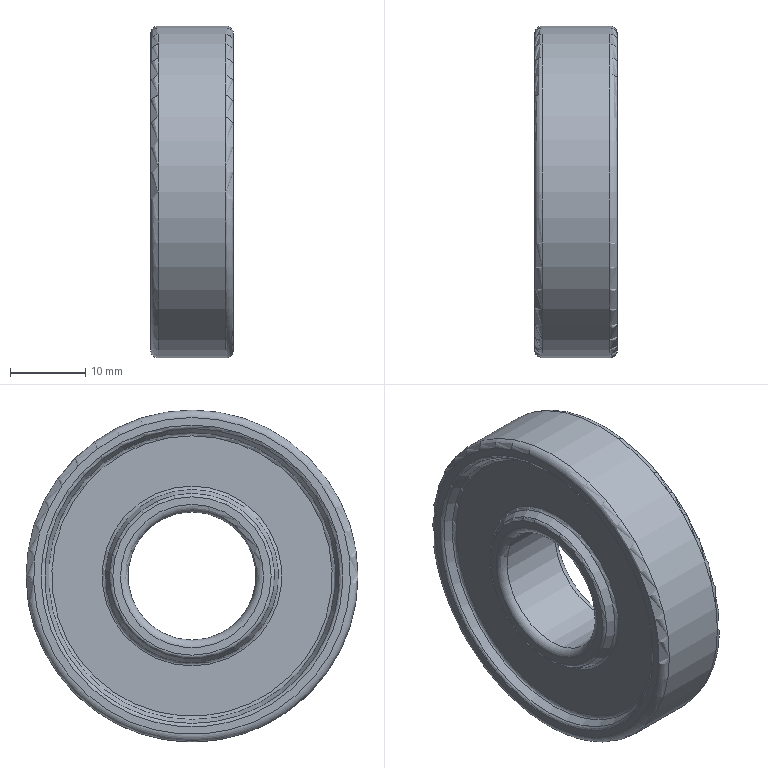Part | STEP file | PL6203ZZA_default | 1 solid | 24 faces | box 11 x 44 x 44 mm | volume 11669 mm3 | torus 12 | plane 6 | cone 4 | cylinder 2 | commonest cylinder face diameters 17 x1 44 x1
STEP:
#1=CARTESIAN_POINT('',(0.,0.,0.));
#2=DIRECTION('',(0.,0.,1.));
#3=DIRECTION('',(1.,0.,0.));
#4=AXIS2_PLACEMENT_3D('',#1,#2,#3);
#5=CARTESIAN_POINT('',(0.,-8.5,21.));
#6=VERTEX_POINT('',#5);
#7=CARTESIAN_POINT('',(0.,-8.5,0.));
#8=DIRECTION('',(-1.,0.,0.));
#9=DIRECTION('',(0.,0.,1.));
#10=AXIS2_PLACEMENT_3D('',#7,#8,#9);
#11=CIRCLE('',#10,21.);
#12=CARTESIAN_POINT('',(1.,-8.5,0.));
#13=DIRECTION('',(-1.,0.,0.));
#14=DIRECTION('',(0.,0.,1.));
#15=AXIS2_PLACEMENT_3D('',#12,#13,#14);
#16=TOROIDAL_SURFACE('',#15,21.,1.);
#17=CARTESIAN_POINT('',(0.,7.854));
#18=DIRECTION('',(1.,0.));
#19=VECTOR('',#18,1.);
#20=LINE('',#17,#19);
#21=(GEOMETRIC_REPRESENTATION_CONTEXT(2)PARAMETRIC_REPRESENTATION_CONTEXT()REPRESENTATION_CONTEXT('',''));
#22=DEFINITIONAL_REPRESENTATION('',(#20),#21);
#23=PCURVE('',#16,#22);
#24=CARTESIAN_POINT('',(0.,11.5,0.));
#25=DIRECTION('',(1.,0.,0.));
#26=DIRECTION('',(0.,0.,-1.));
#27=AXIS2_PLACEMENT_3D('',#24,#25,#26);
#28=PLANE('',#27);
#29=CARTESIAN_POINT('',(-21.,-20.));
#30=CARTESIAN_POINT('',(-21.,16.373));
#31=CARTESIAN_POINT('',(10.5,-1.813));
#32=CARTESIAN_POINT('',(42.,-20.));
#33=CARTESIAN_POINT('',(10.5,-38.187));
#34=CARTESIAN_POINT('',(-21.,-56.373));
#35=CARTESIAN_POINT('',(-21.,-20.));
#36=(BOUNDED_CURVE()B_SPLINE_CURVE(2,(#29,#30,#31,#32,#33,#34,#35),.UNSPECIFIED.,.T.,.F.)B_SPLINE_CURVE_WITH_KNOTS((1,2,2,2,2,1),(-2.094,0.,2.094,4.189,6.283,8.378),.UNSPECIFIED.)CURVE()GEOMETRIC_REPRESENTATION_ITEM()RATIONAL_B_SPLINE_CURVE((1.,0.5,1.,0.5,1.,0.5,1.))REPRESENTATION_ITEM(''));
#37=(GEOMETRIC_REPRESENTATION_CONTEXT(2)PARAMETRIC_REPRESENTATION_CONTEXT()REPRESENTATION_CONTEXT('',''));
#38=DEFINITIONAL_REPRESENTATION('',(#36),#37);
#39=PCURVE('',#28,#38);
#40=SURFACE_CURVE('',#11,(#23,#39),.PCURVE_S1.);
#41=EDGE_CURVE('',#6,#6,#40,.T.);
#42=ORIENTED_EDGE('',*,*,#41,.F.);
#43=CARTESIAN_POINT('',(1.,-8.5,22.));
#44=VERTEX_POINT('',#43);
#45=CARTESIAN_POINT('',(1.,-8.5,22.));
#46=CARTESIAN_POINT('',(0.7327,-8.5,22.));
#47=CARTESIAN_POINT('',(0.4723,-8.5,21.915));
#48=CARTESIAN_POINT('',(0.2481,-8.5,21.752));
#49=CARTESIAN_POINT('',(0.085,-8.5,21.528));
#50=CARTESIAN_POINT('',(0.,-8.5,21.267));
#51=CARTESIAN_POINT('',(0.,-8.5,21.));
#52=(BOUNDED_CURVE()B_SPLINE_CURVE(6,(#45,#46,#47,#48,#49,#50,#51),.UNSPECIFIED.,.F.,.F.)B_SPLINE_CURVE_WITH_KNOTS((7,7),(0.,1.571),.PIECEWISE_BEZIER_KNOTS.)CURVE()GEOMETRIC_REPRESENTATION_ITEM()RATIONAL_B_SPLINE_CURVE((1.031,1.01,0.9979,0.994,0.9979,1.01,1.031))REPRESENTATION_ITEM(''));
#53=CARTESIAN_POINT('',(0.,6.283));
#54=DIRECTION('',(0.,1.));
#55=VECTOR('',#54,1.);
#56=LINE('',#53,#55);
#57=(GEOMETRIC_REPRESENTATION_CONTEXT(2)PARAMETRIC_REPRESENTATION_CONTEXT()REPRESENTATION_CONTEXT('',''));
#58=DEFINITIONAL_REPRESENTATION('',(#56),#57);
#59=PCURVE('',#16,#58);
#60=CARTESIAN_POINT('',(6.283,6.283));
#61=DIRECTION('',(0.,1.));
#62=VECTOR('',#61,1.);
#63=LINE('',#60,#62);
#64=(GEOMETRIC_REPRESENTATION_CONTEXT(2)PARAMETRIC_REPRESENTATION_CONTEXT()REPRESENTATION_CONTEXT('',''));
#65=DEFINITIONAL_REPRESENTATION('',(#63),#64);
#66=PCURVE('',#16,#65);
#67=SEAM_CURVE('',#52,(#59,#66),.PCURVE_S1.);
#68=EDGE_CURVE('',#44,#6,#67,.T.);
#69=ORIENTED_EDGE('',*,*,#68,.F.);
#70=CARTESIAN_POINT('',(1.,-8.5,0.));
#71=DIRECTION('',(-1.,0.,0.));
#72=DIRECTION('',(0.,0.,1.));
#73=AXIS2_PLACEMENT_3D('',#70,#71,#72);
#74=CIRCLE('',#73,22.);
#75=CARTESIAN_POINT('',(0.,6.283));
#76=DIRECTION('',(1.,0.));
#77=VECTOR('',#76,1.);
#78=LINE('',#75,#77);
#79=(GEOMETRIC_REPRESENTATION_CONTEXT(2)PARAMETRIC_REPRESENTATION_CONTEXT()REPRESENTATION_CONTEXT('',''));
#80=DEFINITIONAL_REPRESENTATION('',(#78),#79);
#81=PCURVE('',#16,#80);
#82=CARTESIAN_POINT('',(5.5,-8.5,0.));
#83=DIRECTION('',(-1.,0.,0.));
#84=DIRECTION('',(0.,0.,1.));
#85=AXIS2_PLACEMENT_3D('',#82,#83,#84);
#86=CYLINDRICAL_SURFACE('',#85,22.);
#87=CARTESIAN_POINT('',(0.,4.5));
#88=DIRECTION('',(1.,0.));
#89=VECTOR('',#88,1.);
#90=LINE('',#87,#89);
#91=(GEOMETRIC_REPRESENTATION_CONTEXT(2)PARAMETRIC_REPRESENTATION_CONTEXT()REPRESENTATION_CONTEXT('',''));
#92=DEFINITIONAL_REPRESENTATION('',(#90),#91);
#93=PCURVE('',#86,#92);
#94=SURFACE_CURVE('',#74,(#81,#93),.PCURVE_S1.);
#95=EDGE_CURVE('',#44,#44,#94,.T.);
#96=ORIENTED_EDGE('',*,*,#95,.T.);
#97=ORIENTED_EDGE('',*,*,#68,.T.);
#98=EDGE_LOOP('',(#42,#69,#96,#97));
#99=FACE_BOUND('',#98,.T.);
#100=ADVANCED_FACE('',(#99),#16,.T.);
#101=ORIENTED_EDGE('',*,*,#95,.F.);
#102=CARTESIAN_POINT('',(10.,-8.5,22.));
#103=VERTEX_POINT('',#102);
#104=CARTESIAN_POINT('',(10.,-8.5,22.));
#105=CARTESIAN_POINT('',(1.,-8.5,22.));
#106=B_SPLINE_CURVE_WITH_KNOTS('',1,(#104,#105),.UNSPECIFIED.,.F.,.F.,(2,2),(-4.5,4.5),.PIECEWISE_BEZIER_KNOTS.);
#107=CARTESIAN_POINT('',(0.,0.));
#108=DIRECTION('',(0.,1.));
#109=VECTOR('',#108,1.);
#110=LINE('',#107,#109);
#111=(GEOMETRIC_REPRESENTATION_CONTEXT(2)PARAMETRIC_REPRESENTATION_CONTEXT()REPRESENTATION_CONTEXT('',''));
#112=DEFINITIONAL_REPRESENTATION('',(#110),#111);
#113=PCURVE('',#86,#112);
#114=CARTESIAN_POINT('',(6.283,0.));
#115=DIRECTION('',(0.,1.));
#116=VECTOR('',#115,1.);
#117=LINE('',#114,#116);
#118=(GEOMETRIC_REPRESENTATION_CONTEXT(2)PARAMETRIC_REPRESENTATION_CONTEXT()REPRESENTATION_CONTEXT('',''));
#119=DEFINITIONAL_REPRESENTATION('',(#117),#118);
#120=PCURVE('',#86,#119);
#121=SEAM_CURVE('',#106,(#113,#120),.PCURVE_S1.);
#122=EDGE_CURVE('',#103,#44,#121,.T.);
#123=ORIENTED_EDGE('',*,*,#122,.F.);
#124=CARTESIAN_POINT('',(10.,-8.5,0.));
#125=DIRECTION('',(-1.,0.,0.));
#126=DIRECTION('',(0.,0.,1.));
#127=AXIS2_PLACEMENT_3D('',#124,#125,#126);
#128=CIRCLE('',#127,22.);
#129=CARTESIAN_POINT('',(0.,-4.5));
#130=DIRECTION('',(1.,0.));
#131=VECTOR('',#130,1.);
#132=LINE('',#129,#131);
#133=(GEOMETRIC_REPRESENTATION_CONTEXT(2)PARAMETRIC_REPRESENTATION_CONTEXT()REPRESENTATION_CONTEXT('',''));
#134=DEFINITIONAL_REPRESENTATION('',(#132),#133);
#135=PCURVE('',#86,#134);
#136=CARTESIAN_POINT('',(10.,-8.5,0.));
#137=DIRECTION('',(-1.,0.,0.));
#138=DIRECTION('',(0.,0.,1.));
#139=AXIS2_PLACEMENT_3D('',#136,#137,#138);
#140=TOROIDAL_SURFACE('',#139,21.,1.);
#141=CARTESIAN_POINT('',(0.,6.283));
#142=DIRECTION('',(1.,0.));
#143=VECTOR('',#142,1.);
#144=LINE('',#141,#143);
#145=(GEOMETRIC_REPRESENTATION_CONTEXT(2)PARAMETRIC_REPRESENTATION_CONTEXT()REPRESENTATION_CONTEXT('',''));
#146=DEFINITIONAL_REPRESENTATION('',(#144),#145);
#147=PCURVE('',#140,#146);
#148=SURFACE_CURVE('',#128,(#135,#147),.PCURVE_S1.);
#149=EDGE_CURVE('',#103,#103,#148,.T.);
#150=ORIENTED_EDGE('',*,*,#149,.T.);
#151=ORIENTED_EDGE('',*,*,#122,.T.);
#152=EDGE_LOOP('',(#101,#123,#150,#151));
#153=FACE_BOUND('',#152,.T.);
#154=ADVANCED_FACE('',(#153),#86,.T.);
#155=ORIENTED_EDGE('',*,*,#149,.F.);
#156=CARTESIAN_POINT('',(11.,-8.5,21.));
#157=VERTEX_POINT('',#156);
#158=CARTESIAN_POINT('',(11.,-8.5,21.));
#159=CARTESIAN_POINT('',(11.,-8.5,21.267));
#160=CARTESIAN_POINT('',(10.915,-8.5,21.528));
#161=CARTESIAN_POINT('',(10.752,-8.5,21.752));
#162=CARTESIAN_POINT('',(10.528,-8.5,21.915));
#163=CARTESIAN_POINT('',(10.267,-8.5,22.));
#164=CARTESIAN_POINT('',(10.,-8.5,22.));
#165=(BOUNDED_CURVE()B_SPLINE_CURVE(6,(#158,#159,#160,#161,#162,#163,#164),.UNSPECIFIED.,.F.,.F.)B_SPLINE_CURVE_WITH_KNOTS((7,7),(-1.571,0.),.PIECEWISE_BEZIER_KNOTS.)CURVE()GEOMETRIC_REPRESENTATION_ITEM()RATIONAL_B_SPLINE_CURVE((1.031,1.01,0.9979,0.994,0.9979,1.01,1.031))REPRESENTATION_ITEM(''));
#166=CARTESIAN_POINT('',(0.,6.283));
#167=DIRECTION('',(0.,1.));
#168=VECTOR('',#167,1.);
#169=LINE('',#166,#168);
#170=(GEOMETRIC_REPRESENTATION_CONTEXT(2)PARAMETRIC_REPRESENTATION_CONTEXT()REPRESENTATION_CONTEXT('',''));
#171=DEFINITIONAL_REPRESENTATION('',(#169),#170);
#172=PCURVE('',#140,#171);
#173=CARTESIAN_POINT('',(6.283,6.283));
#174=DIRECTION('',(0.,1.));
#175=VECTOR('',#174,1.);
#176=LINE('',#173,#175);
#177=(GEOMETRIC_REPRESENTATION_CONTEXT(2)PARAMETRIC_REPRESENTATION_CONTEXT()REPRESENTATION_CONTEXT('',''));
#178=DEFINITIONAL_REPRESENTATION('',(#176),#177);
#179=PCURVE('',#140,#178);
#180=SEAM_CURVE('',#165,(#172,#179),.PCURVE_S1.);
#181=EDGE_CURVE('',#157,#103,#180,.T.);
#182=ORIENTED_EDGE('',*,*,#181,.F.);
#183=CARTESIAN_POINT('',(11.,-8.5,0.));
#184=DIRECTION('',(-1.,0.,0.));
#185=DIRECTION('',(0.,0.,1.));
#186=AXIS2_PLACEMENT_3D('',#183,#184,#185);
#187=CIRCLE('',#186,21.);
#188=CARTESIAN_POINT('',(0.,4.712));
#189=DIRECTION('',(1.,0.));
#190=VECTOR('',#189,1.);
#191=LINE('',#188,#190);
#192=(GEOMETRIC_REPRESENTATION_CONTEXT(2)PARAMETRIC_REPRESENTATION_CONTEXT()REPRESENTATION_CONTEXT('',''));
#193=DEFINITIONAL_REPRESENTATION('',(#191),#192);
#194=PCURVE('',#140,#193);
#195=CARTESIAN_POINT('',(11.,12.5,0.));
#196=DIRECTION('',(-1.,0.,0.));
#197=DIRECTION('',(0.,0.,1.));
#198=AXIS2_PLACEMENT_3D('',#195,#196,#197);
#199=PLANE('',#198);
#200=CARTESIAN_POINT('',(0.,-21.));
#201=DIRECTION('',(1.,0.));
#202=AXIS2_PLACEMENT_2D('',#200,#201);
#203=CIRCLE('',#202,21.);
#204=(GEOMETRIC_REPRESENTATION_CONTEXT(2)PARAMETRIC_REPRESENTATION_CONTEXT()REPRESENTATION_CONTEXT('',''));
#205=DEFINITIONAL_REPRESENTATION('',(#203),#204);
#206=PCURVE('',#199,#205);
#207=SURFACE_CURVE('',#187,(#194,#206),.PCURVE_S1.);
#208=EDGE_CURVE('',#157,#157,#207,.T.);
#209=ORIENTED_EDGE('',*,*,#208,.T.);
#210=ORIENTED_EDGE('',*,*,#181,.T.);
#211=EDGE_LOOP('',(#155,#182,#209,#210));
#212=FACE_BOUND('',#211,.T.);
#213=ADVANCED_FACE('',(#212),#140,.T.);
#214=ORIENTED_EDGE('',*,*,#208,.F.);
#215=EDGE_LOOP('',(#214));
#216=FACE_BOUND('',#215,.T.);
#217=CARTESIAN_POINT('',(11.,-8.5,20.));
#218=VERTEX_POINT('',#217);
#219=CARTESIAN_POINT('',(11.,-8.5,0.));
#220=DIRECTION('',(-1.,0.,0.));
#221=DIRECTION('',(0.,0.,1.));
#222=AXIS2_PLACEMENT_3D('',#219,#220,#221);
#223=CIRCLE('',#222,20.);
#224=CARTESIAN_POINT('',(0.,-21.));
#225=DIRECTION('',(1.,0.));
#226=AXIS2_PLACEMENT_2D('',#224,#225);
#227=CIRCLE('',#226,20.);
#228=(GEOMETRIC_REPRESENTATION_CONTEXT(2)PARAMETRIC_REPRESENTATION_CONTEXT()REPRESENTATION_CONTEXT('',''));
#229=DEFINITIONAL_REPRESENTATION('',(#227),#228);
#230=PCURVE('',#199,#229);
#231=CARTESIAN_POINT('',(10.5,-8.5,0.));
#232=DIRECTION('',(-1.,0.,0.));
#233=DIRECTION('',(0.,0.,1.));
#234=AXIS2_PLACEMENT_3D('',#231,#232,#233);
#235=TOROIDAL_SURFACE('',#234,20.,0.5);
#236=CARTESIAN_POINT('',(0.,4.712));
#237=DIRECTION('',(1.,0.));
#238=VECTOR('',#237,1.);
#239=LINE('',#236,#238);
#240=(GEOMETRIC_REPRESENTATION_CONTEXT(2)PARAMETRIC_REPRESENTATION_CONTEXT()REPRESENTATION_CONTEXT('',''));
#241=DEFINITIONAL_REPRESENTATION('',(#239),#240);
#242=PCURVE('',#235,#241);
#243=SURFACE_CURVE('',#223,(#230,#242),.PCURVE_S1.);
#244=EDGE_CURVE('',#218,#218,#243,.T.);
#245=ORIENTED_EDGE('',*,*,#244,.T.);
#246=EDGE_LOOP('',(#245));
#247=FACE_BOUND('',#246,.T.);
#248=ADVANCED_FACE('',(#216,#247),#199,.F.);
#249=ORIENTED_EDGE('',*,*,#244,.F.);
#250=CARTESIAN_POINT('',(10.724,-8.5,19.553));
#251=VERTEX_POINT('',#250);
#252=CARTESIAN_POINT('',(10.724,-8.5,19.553));
#253=CARTESIAN_POINT('',(10.807,-8.5,19.594));
#254=CARTESIAN_POINT('',(10.88,-8.5,19.654));
#255=CARTESIAN_POINT('',(10.939,-8.5,19.729));
#256=CARTESIAN_POINT('',(10.979,-8.5,19.815));
#257=CARTESIAN_POINT('',(11.,-8.5,19.907));
#258=CARTESIAN_POINT('',(11.,-8.5,20.));
#259=(BOUNDED_CURVE()B_SPLINE_CURVE(6,(#252,#253,#254,#255,#256,#257,#258),.UNSPECIFIED.,.F.,.F.)B_SPLINE_CURVE_WITH_KNOTS((7,7),(3.605,4.712),.PIECEWISE_BEZIER_KNOTS.)CURVE()GEOMETRIC_REPRESENTATION_ITEM()RATIONAL_B_SPLINE_CURVE((1.015,1.005,0.999,0.997,0.999,1.005,1.015))REPRESENTATION_ITEM(''));
#260=CARTESIAN_POINT('',(0.,0.));
#261=DIRECTION('',(0.,1.));
#262=VECTOR('',#261,1.);
#263=LINE('',#260,#262);
#264=(GEOMETRIC_REPRESENTATION_CONTEXT(2)PARAMETRIC_REPRESENTATION_CONTEXT()REPRESENTATION_CONTEXT('',''));
#265=DEFINITIONAL_REPRESENTATION('',(#263),#264);
#266=PCURVE('',#235,#265);
#267=CARTESIAN_POINT('',(6.283,0.));
#268=DIRECTION('',(0.,1.));
#269=VECTOR('',#268,1.);
#270=LINE('',#267,#269);
#271=(GEOMETRIC_REPRESENTATION_CONTEXT(2)PARAMETRIC_REPRESENTATION_CONTEXT()REPRESENTATION_CONTEXT('',''));
#272=DEFINITIONAL_REPRESENTATION('',(#270),#271);
#273=PCURVE('',#235,#272);
#274=SEAM_CURVE('',#259,(#266,#273),.PCURVE_S1.);
#275=EDGE_CURVE('',#251,#218,#274,.T.);
#276=ORIENTED_EDGE('',*,*,#275,.F.);
#277=CARTESIAN_POINT('',(10.724,-8.5,0.));
#278=DIRECTION('',(-1.,0.,0.));
#279=DIRECTION('',(0.,0.,1.));
#280=AXIS2_PLACEMENT_3D('',#277,#278,#279);
#281=CIRCLE('',#280,19.553);
#282=CARTESIAN_POINT('',(0.,3.605));
#283=DIRECTION('',(1.,0.));
#284=VECTOR('',#283,1.);
#285=LINE('',#282,#284);
#286=(GEOMETRIC_REPRESENTATION_CONTEXT(2)PARAMETRIC_REPRESENTATION_CONTEXT()REPRESENTATION_CONTEXT('',''));
#287=DEFINITIONAL_REPRESENTATION('',(#285),#286);
#288=PCURVE('',#235,#287);
#289=CARTESIAN_POINT('',(9.676,-8.5,0.));
#290=DIRECTION('',(1.,0.,0.));
#291=DIRECTION('',(0.,0.,-1.));
#292=AXIS2_PLACEMENT_3D('',#289,#290,#291);
#293=CONICAL_SURFACE('',#292,19.029,0.4636);
#294=CARTESIAN_POINT('',(9.425,1.047));
#295=DIRECTION('',(-1.,0.));
#296=VECTOR('',#295,1.);
#297=LINE('',#294,#296);
#298=(GEOMETRIC_REPRESENTATION_CONTEXT(2)PARAMETRIC_REPRESENTATION_CONTEXT()REPRESENTATION_CONTEXT('',''));
#299=DEFINITIONAL_REPRESENTATION('',(#297),#298);
#300=PCURVE('',#293,#299);
#301=SURFACE_CURVE('',#281,(#288,#300),.PCURVE_S1.);
#302=EDGE_CURVE('',#251,#251,#301,.T.);
#303=ORIENTED_EDGE('',*,*,#302,.T.);
#304=ORIENTED_EDGE('',*,*,#275,.T.);
#305=EDGE_LOOP('',(#249,#276,#303,#304));
#306=FACE_BOUND('',#305,.T.);
#307=ADVANCED_FACE('',(#306),#235,.T.);
#308=ORIENTED_EDGE('',*,*,#302,.T.);
#309=CARTESIAN_POINT('',(9.676,-8.5,19.029));
#310=VERTEX_POINT('',#309);
#311=CARTESIAN_POINT('',(9.676,-8.5,19.029));
#312=CARTESIAN_POINT('',(10.724,-8.5,19.553));
#313=B_SPLINE_CURVE_WITH_KNOTS('',1,(#311,#312),.UNSPECIFIED.,.F.,.F.,(2,2),(0.,1.171),.PIECEWISE_BEZIER_KNOTS.);
#314=CARTESIAN_POINT('',(3.142,0.));
#315=DIRECTION('',(0.,1.));
#316=VECTOR('',#315,1.);
#317=LINE('',#314,#316);
#318=(GEOMETRIC_REPRESENTATION_CONTEXT(2)PARAMETRIC_REPRESENTATION_CONTEXT()REPRESENTATION_CONTEXT('',''));
#319=DEFINITIONAL_REPRESENTATION('',(#317),#318);
#320=PCURVE('',#293,#319);
#321=CARTESIAN_POINT('',(9.425,0.));
#322=DIRECTION('',(0.,1.));
#323=VECTOR('',#322,1.);
#324=LINE('',#321,#323);
#325=(GEOMETRIC_REPRESENTATION_CONTEXT(2)PARAMETRIC_REPRESENTATION_CONTEXT()REPRESENTATION_CONTEXT('',''));
#326=DEFINITIONAL_REPRESENTATION('',(#324),#325);
#327=PCURVE('',#293,#326);
#328=SEAM_CURVE('',#313,(#320,#327),.PCURVE_S1.);
#329=EDGE_CURVE('',#310,#251,#328,.T.);
#330=ORIENTED_EDGE('',*,*,#329,.F.);
#331=CARTESIAN_POINT('',(9.676,-8.5,0.));
#332=DIRECTION('',(-1.,0.,0.));
#333=DIRECTION('',(0.,0.,1.));
#334=AXIS2_PLACEMENT_3D('',#331,#332,#333);
#335=CIRCLE('',#334,19.029);
#336=CARTESIAN_POINT('',(9.425,0.));
#337=DIRECTION('',(-1.,0.));
#338=VECTOR('',#337,1.);
#339=LINE('',#336,#338);
#340=(GEOMETRIC_REPRESENTATION_CONTEXT(2)PARAMETRIC_REPRESENTATION_CONTEXT()REPRESENTATION_CONTEXT('',''));
#341=DEFINITIONAL_REPRESENTATION('',(#339),#340);
#342=PCURVE('',#293,#341);
#343=CARTESIAN_POINT('',(9.9,-8.5,0.));
#344=DIRECTION('',(-1.,0.,0.));
#345=DIRECTION('',(0.,0.,1.));
#346=AXIS2_PLACEMENT_3D('',#343,#344,#345);
#347=TOROIDAL_SURFACE('',#346,18.582,0.5);
#348=CARTESIAN_POINT('',(0.,6.747));
#349=DIRECTION('',(1.,0.));
#350=VECTOR('',#349,1.);
#351=LINE('',#348,#350);
#352=(GEOMETRIC_REPRESENTATION_CONTEXT(2)PARAMETRIC_REPRESENTATION_CONTEXT()REPRESENTATION_CONTEXT('',''));
#353=DEFINITIONAL_REPRESENTATION('',(#351),#352);
#354=PCURVE('',#347,#353);
#355=SURFACE_CURVE('',#335,(#342,#354),.PCURVE_S1.);
#356=EDGE_CURVE('',#310,#310,#355,.T.);
#357=ORIENTED_EDGE('',*,*,#356,.F.);
#358=ORIENTED_EDGE('',*,*,#329,.T.);
#359=EDGE_LOOP('',(#308,#330,#357,#358));
#360=FACE_BOUND('',#359,.F.);
#361=ADVANCED_FACE('',(#360),#293,.F.);
#362=ORIENTED_EDGE('',*,*,#356,.T.);
#363=CARTESIAN_POINT('',(9.4,-8.5,18.582));
#364=VERTEX_POINT('',#363);
#365=CARTESIAN_POINT('',(9.676,-8.5,19.029));
#366=CARTESIAN_POINT('',(9.593,-8.5,18.987));
#367=CARTESIAN_POINT('',(9.52,-8.5,18.928));
#368=CARTESIAN_POINT('',(9.461,-8.5,18.853));
#369=CARTESIAN_POINT('',(9.421,-8.5,18.767));
#370=CARTESIAN_POINT('',(9.4,-8.5,18.675));
#371=CARTESIAN_POINT('',(9.4,-8.5,18.582));
#372=(BOUNDED_CURVE()B_SPLINE_CURVE(6,(#365,#366,#367,#368,#369,#370,#371),.UNSPECIFIED.,.F.,.F.)B_SPLINE_CURVE_WITH_KNOTS((7,7),(0.4636,1.571),.PIECEWISE_BEZIER_KNOTS.)CURVE()GEOMETRIC_REPRESENTATION_ITEM()RATIONAL_B_SPLINE_CURVE((1.015,1.005,0.999,0.997,0.999,1.005,1.015))REPRESENTATION_ITEM(''));
#373=CARTESIAN_POINT('',(6.283,6.283));
#374=DIRECTION('',(0.,1.));
#375=VECTOR('',#374,1.);
#376=LINE('',#373,#375);
#377=(GEOMETRIC_REPRESENTATION_CONTEXT(2)PARAMETRIC_REPRESENTATION_CONTEXT()REPRESENTATION_CONTEXT('',''));
#378=DEFINITIONAL_REPRESENTATION('',(#376),#377);
#379=PCURVE('',#347,#378);
#380=CARTESIAN_POINT('',(0.,6.283));
#381=DIRECTION('',(0.,1.));
#382=VECTOR('',#381,1.);
#383=LINE('',#380,#382);
#384=(GEOMETRIC_REPRESENTATION_CONTEXT(2)PARAMETRIC_REPRESENTATION_CONTEXT()REPRESENTATION_CONTEXT('',''));
#385=DEFINITIONAL_REPRESENTATION('',(#383),#384);
#386=PCURVE('',#347,#385);
#387=SEAM_CURVE('',#372,(#379,#386),.PCURVE_S1.);
#388=EDGE_CURVE('',#310,#364,#387,.T.);
#389=ORIENTED_EDGE('',*,*,#388,.T.);
#390=CARTESIAN_POINT('',(9.4,-8.5,0.));
#391=DIRECTION('',(-1.,0.,0.));
#392=DIRECTION('',(0.,0.,1.));
#393=AXIS2_PLACEMENT_3D('',#390,#391,#392);
#394=CIRCLE('',#393,18.582);
#395=CARTESIAN_POINT('',(0.,7.854));
#396=DIRECTION('',(1.,0.));
#397=VECTOR('',#396,1.);
#398=LINE('',#395,#397);
#399=(GEOMETRIC_REPRESENTATION_CONTEXT(2)PARAMETRIC_REPRESENTATION_CONTEXT()REPRESENTATION_CONTEXT('',''));
#400=DEFINITIONAL_REPRESENTATION('',(#398),#399);
#401=PCURVE('',#347,#400);
#402=CARTESIAN_POINT('',(9.4,10.082,0.));
#403=DIRECTION('',(-1.,0.,0.));
#404=DIRECTION('',(0.,0.,1.));
#405=AXIS2_PLACEMENT_3D('',#402,#403,#404);
#406=PLANE('',#405);
#407=CARTESIAN_POINT('',(0.,-18.582));
#408=DIRECTION('',(1.,0.));
#409=AXIS2_PLACEMENT_2D('',#407,#408);
#410=CIRCLE('',#409,18.582);
#411=(GEOMETRIC_REPRESENTATION_CONTEXT(2)PARAMETRIC_REPRESENTATION_CONTEXT()REPRESENTATION_CONTEXT('',''));
#412=DEFINITIONAL_REPRESENTATION('',(#410),#411);
#413=PCURVE('',#406,#412);
#414=SURFACE_CURVE('',#394,(#401,#413),.PCURVE_S1.);
#415=EDGE_CURVE('',#364,#364,#414,.T.);
#416=ORIENTED_EDGE('',*,*,#415,.F.);
#417=ORIENTED_EDGE('',*,*,#388,.F.);
#418=EDGE_LOOP('',(#362,#389,#416,#417));
#419=FACE_BOUND('',#418,.F.);
#420=ADVANCED_FACE('',(#419),#347,.F.);
#421=ORIENTED_EDGE('',*,*,#415,.F.);
#422=EDGE_LOOP('',(#421));
#423=FACE_BOUND('',#422,.T.);
#424=CARTESIAN_POINT('',(9.4,-8.5,11.918));
#425=VERTEX_POINT('',#424);
#426=CARTESIAN_POINT('',(9.4,-8.5,0.));
#427=DIRECTION('',(-1.,0.,0.));
#428=DIRECTION('',(0.,0.,1.));
#429=AXIS2_PLACEMENT_3D('',#426,#427,#428);
#430=CIRCLE('',#429,11.918);
#431=CARTESIAN_POINT('',(0.,-18.582));
#432=DIRECTION('',(1.,0.));
#433=AXIS2_PLACEMENT_2D('',#431,#432);
#434=CIRCLE('',#433,11.918);
#435=(GEOMETRIC_REPRESENTATION_CONTEXT(2)PARAMETRIC_REPRESENTATION_CONTEXT()REPRESENTATION_CONTEXT('',''));
#436=DEFINITIONAL_REPRESENTATION('',(#434),#435);
#437=PCURVE('',#406,#436);
#438=CARTESIAN_POINT('',(9.9,-8.5,0.));
#439=DIRECTION('',(-1.,0.,0.));
#440=DIRECTION('',(0.,0.,1.));
#441=AXIS2_PLACEMENT_3D('',#438,#439,#440);
#442=TOROIDAL_SURFACE('',#441,11.918,0.5);
#443=CARTESIAN_POINT('',(0.,7.854));
#444=DIRECTION('',(1.,0.));
#445=VECTOR('',#444,1.);
#446=LINE('',#443,#445);
#447=(GEOMETRIC_REPRESENTATION_CONTEXT(2)PARAMETRIC_REPRESENTATION_CONTEXT()REPRESENTATION_CONTEXT('',''));
#448=DEFINITIONAL_REPRESENTATION('',(#446),#447);
#449=PCURVE('',#442,#448);
#450=SURFACE_CURVE('',#430,(#437,#449),.PCURVE_S1.);
#451=EDGE_CURVE('',#425,#425,#450,.T.);
#452=ORIENTED_EDGE('',*,*,#451,.T.);
#453=EDGE_LOOP('',(#452));
#454=FACE_BOUND('',#453,.T.);
#455=ADVANCED_FACE('',(#423,#454),#406,.F.);
#456=ORIENTED_EDGE('',*,*,#451,.T.);
#457=CARTESIAN_POINT('',(9.676,-8.5,11.471));
#458=VERTEX_POINT('',#457);
#459=CARTESIAN_POINT('',(9.4,-8.5,11.918));
#460=CARTESIAN_POINT('',(9.4,-8.5,11.825));
#461=CARTESIAN_POINT('',(9.421,-8.5,11.733));
#462=CARTESIAN_POINT('',(9.461,-8.5,11.647));
#463=CARTESIAN_POINT('',(9.52,-8.5,11.572));
#464=CARTESIAN_POINT('',(9.593,-8.5,11.513));
#465=CARTESIAN_POINT('',(9.676,-8.5,11.471));
#466=(BOUNDED_CURVE()B_SPLINE_CURVE(6,(#459,#460,#461,#462,#463,#464,#465),.UNSPECIFIED.,.F.,.F.)B_SPLINE_CURVE_WITH_KNOTS((7,7),(1.571,2.678),.PIECEWISE_BEZIER_KNOTS.)CURVE()GEOMETRIC_REPRESENTATION_ITEM()RATIONAL_B_SPLINE_CURVE((1.015,1.005,0.999,0.997,0.999,1.005,1.015))REPRESENTATION_ITEM(''));
#467=CARTESIAN_POINT('',(6.283,6.283));
#468=DIRECTION('',(0.,1.));
#469=VECTOR('',#468,1.);
#470=LINE('',#467,#469);
#471=(GEOMETRIC_REPRESENTATION_CONTEXT(2)PARAMETRIC_REPRESENTATION_CONTEXT()REPRESENTATION_CONTEXT('',''));
#472=DEFINITIONAL_REPRESENTATION('',(#470),#471);
#473=PCURVE('',#442,#472);
#474=CARTESIAN_POINT('',(0.,6.283));
#475=DIRECTION('',(0.,1.));
#476=VECTOR('',#475,1.);
#477=LINE('',#474,#476);
#478=(GEOMETRIC_REPRESENTATION_CONTEXT(2)PARAMETRIC_REPRESENTATION_CONTEXT()REPRESENTATION_CONTEXT('',''));
#479=DEFINITIONAL_REPRESENTATION('',(#477),#478);
#480=PCURVE('',#442,#479);
#481=SEAM_CURVE('',#466,(#473,#480),.PCURVE_S1.);
#482=EDGE_CURVE('',#425,#458,#481,.T.);
#483=ORIENTED_EDGE('',*,*,#482,.T.);
#484=CARTESIAN_POINT('',(9.676,-8.5,0.));
#485=DIRECTION('',(-1.,0.,0.));
#486=DIRECTION('',(0.,0.,1.));
#487=AXIS2_PLACEMENT_3D('',#484,#485,#486);
#488=CIRCLE('',#487,11.471);
#489=CARTESIAN_POINT('',(0.,8.961));
#490=DIRECTION('',(1.,0.));
#491=VECTOR('',#490,1.);
#492=LINE('',#489,#491);
#493=(GEOMETRIC_REPRESENTATION_CONTEXT(2)PARAMETRIC_REPRESENTATION_CONTEXT()REPRESENTATION_CONTEXT('',''));
#494=DEFINITIONAL_REPRESENTATION('',(#492),#493);
#495=PCURVE('',#442,#494);
#496=CARTESIAN_POINT('',(10.724,-8.5,0.));
#497=DIRECTION('',(-1.,0.,0.));
#498=DIRECTION('',(0.,0.,1.));
#499=AXIS2_PLACEMENT_3D('',#496,#497,#498);
#500=CONICAL_SURFACE('',#499,10.947,0.4636);
#501=CARTESIAN_POINT('',(0.,1.047));
#502=DIRECTION('',(1.,0.));
#503=VECTOR('',#502,1.);
#504=LINE('',#501,#503);
#505=(GEOMETRIC_REPRESENTATION_CONTEXT(2)PARAMETRIC_REPRESENTATION_CONTEXT()REPRESENTATION_CONTEXT('',''));
#506=DEFINITIONAL_REPRESENTATION('',(#504),#505);
#507=PCURVE('',#500,#506);
#508=SURFACE_CURVE('',#488,(#495,#507),.PCURVE_S1.);
#509=EDGE_CURVE('',#458,#458,#508,.T.);
#510=ORIENTED_EDGE('',*,*,#509,.F.);
#511=ORIENTED_EDGE('',*,*,#482,.F.);
#512=EDGE_LOOP('',(#456,#483,#510,#511));
#513=FACE_BOUND('',#512,.F.);
#514=ADVANCED_FACE('',(#513),#442,.F.);
#515=ORIENTED_EDGE('',*,*,#509,.F.);
#516=CARTESIAN_POINT('',(10.724,-8.5,10.947));
#517=VERTEX_POINT('',#516);
#518=CARTESIAN_POINT('',(10.724,-8.5,10.947));
#519=CARTESIAN_POINT('',(9.676,-8.5,11.471));
#520=B_SPLINE_CURVE_WITH_KNOTS('',1,(#518,#519),.UNSPECIFIED.,.F.,.F.,(2,2),(0.,1.171),.PIECEWISE_BEZIER_KNOTS.);
#521=CARTESIAN_POINT('',(0.,0.));
#522=DIRECTION('',(0.,1.));
#523=VECTOR('',#522,1.);
#524=LINE('',#521,#523);
#525=(GEOMETRIC_REPRESENTATION_CONTEXT(2)PARAMETRIC_REPRESENTATION_CONTEXT()REPRESENTATION_CONTEXT('',''));
#526=DEFINITIONAL_REPRESENTATION('',(#524),#525);
#527=PCURVE('',#500,#526);
#528=CARTESIAN_POINT('',(6.283,0.));
#529=DIRECTION('',(0.,1.));
#530=VECTOR('',#529,1.);
#531=LINE('',#528,#530);
#532=(GEOMETRIC_REPRESENTATION_CONTEXT(2)PARAMETRIC_REPRESENTATION_CONTEXT()REPRESENTATION_CONTEXT('',''));
#533=DEFINITIONAL_REPRESENTATION('',(#531),#532);
#534=PCURVE('',#500,#533);
#535=SEAM_CURVE('',#520,(#527,#534),.PCURVE_S1.);
#536=EDGE_CURVE('',#517,#458,#535,.T.);
#537=ORIENTED_EDGE('',*,*,#536,.F.);
#538=CARTESIAN_POINT('',(10.724,-8.5,0.));
#539=DIRECTION('',(-1.,0.,0.));
#540=DIRECTION('',(0.,0.,1.));
#541=AXIS2_PLACEMENT_3D('',#538,#539,#540);
#542=CIRCLE('',#541,10.947);
#543=CARTESIAN_POINT('',(0.,0.));
#544=DIRECTION('',(1.,0.));
#545=VECTOR('',#544,1.);
#546=LINE('',#543,#545);
#547=(GEOMETRIC_REPRESENTATION_CONTEXT(2)PARAMETRIC_REPRESENTATION_CONTEXT()REPRESENTATION_CONTEXT('',''));
#548=DEFINITIONAL_REPRESENTATION('',(#546),#547);
#549=PCURVE('',#500,#548);
#550=CARTESIAN_POINT('',(10.5,-8.5,0.));
#551=DIRECTION('',(-1.,0.,0.));
#552=DIRECTION('',(0.,0.,1.));
#553=AXIS2_PLACEMENT_3D('',#550,#551,#552);
#554=TOROIDAL_SURFACE('',#553,10.5,0.5);
#555=CARTESIAN_POINT('',(0.,5.82));
#556=DIRECTION('',(1.,0.));
#557=VECTOR('',#556,1.);
#558=LINE('',#555,#557);
#559=(GEOMETRIC_REPRESENTATION_CONTEXT(2)PARAMETRIC_REPRESENTATION_CONTEXT()REPRESENTATION_CONTEXT('',''));
#560=DEFINITIONAL_REPRESENTATION('',(#558),#559);
#561=PCURVE('',#554,#560);
#562=SURFACE_CURVE('',#542,(#549,#561),.PCURVE_S1.);
#563=EDGE_CURVE('',#517,#517,#562,.T.);
#564=ORIENTED_EDGE('',*,*,#563,.T.);
#565=ORIENTED_EDGE('',*,*,#536,.T.);
#566=EDGE_LOOP('',(#515,#537,#564,#565));
#567=FACE_BOUND('',#566,.T.);
#568=ADVANCED_FACE('',(#567),#500,.T.);
#569=ORIENTED_EDGE('',*,*,#563,.F.);
#570=CARTESIAN_POINT('',(11.,-8.5,10.5));
#571=VERTEX_POINT('',#570);
#572=CARTESIAN_POINT('',(11.,-8.5,10.5));
#573=CARTESIAN_POINT('',(11.,-8.5,10.593));
#574=CARTESIAN_POINT('',(10.979,-8.5,10.685));
#575=CARTESIAN_POINT('',(10.939,-8.5,10.771));
#576=CARTESIAN_POINT('',(10.88,-8.5,10.846));
#577=CARTESIAN_POINT('',(10.807,-8.5,10.906));
#578=CARTESIAN_POINT('',(10.724,-8.5,10.947));
#579=(BOUNDED_CURVE()B_SPLINE_CURVE(6,(#572,#573,#574,#575,#576,#577,#578),.UNSPECIFIED.,.F.,.F.)B_SPLINE_CURVE_WITH_KNOTS((7,7),(4.712,5.82),.PIECEWISE_BEZIER_KNOTS.)CURVE()GEOMETRIC_REPRESENTATION_ITEM()RATIONAL_B_SPLINE_CURVE((1.015,1.005,0.999,0.997,0.999,1.005,1.015))REPRESENTATION_ITEM(''));
#580=CARTESIAN_POINT('',(0.,0.));
#581=DIRECTION('',(0.,1.));
#582=VECTOR('',#581,1.);
#583=LINE('',#580,#582);
#584=(GEOMETRIC_REPRESENTATION_CONTEXT(2)PARAMETRIC_REPRESENTATION_CONTEXT()REPRESENTATION_CONTEXT('',''));
#585=DEFINITIONAL_REPRESENTATION('',(#583),#584);
#586=PCURVE('',#554,#585);
#587=CARTESIAN_POINT('',(6.283,0.));
#588=DIRECTION('',(0.,1.));
#589=VECTOR('',#588,1.);
#590=LINE('',#587,#589);
#591=(GEOMETRIC_REPRESENTATION_CONTEXT(2)PARAMETRIC_REPRESENTATION_CONTEXT()REPRESENTATION_CONTEXT('',''));
#592=DEFINITIONAL_REPRESENTATION('',(#590),#591);
#593=PCURVE('',#554,#592);
#594=SEAM_CURVE('',#579,(#586,#593),.PCURVE_S1.);
#595=EDGE_CURVE('',#571,#517,#594,.T.);
#596=ORIENTED_EDGE('',*,*,#595,.F.);
#597=CARTESIAN_POINT('',(11.,-8.5,0.));
#598=DIRECTION('',(-1.,0.,0.));
#599=DIRECTION('',(0.,0.,1.));
#600=AXIS2_PLACEMENT_3D('',#597,#598,#599);
#601=CIRCLE('',#600,10.5);
#602=CARTESIAN_POINT('',(0.,4.712));
#603=DIRECTION('',(1.,0.));
#604=VECTOR('',#603,1.);
#605=LINE('',#602,#604);
#606=(GEOMETRIC_REPRESENTATION_CONTEXT(2)PARAMETRIC_REPRESENTATION_CONTEXT()REPRESENTATION_CONTEXT('',''));
#607=DEFINITIONAL_REPRESENTATION('',(#605),#606);
#608=PCURVE('',#554,#607);
#609=CARTESIAN_POINT('',(11.,2.,0.));
#610=DIRECTION('',(-1.,0.,0.));
#611=DIRECTION('',(0.,0.,1.));
#612=AXIS2_PLACEMENT_3D('',#609,#610,#611);
#613=PLANE('',#612);
#614=CARTESIAN_POINT('',(0.,-10.5));
#615=DIRECTION('',(1.,0.));
#616=AXIS2_PLACEMENT_2D('',#614,#615);
#617=CIRCLE('',#616,10.5);
#618=(GEOMETRIC_REPRESENTATION_CONTEXT(2)PARAMETRIC_REPRESENTATION_CONTEXT()REPRESENTATION_CONTEXT('',''));
#619=DEFINITIONAL_REPRESENTATION('',(#617),#618);
#620=PCURVE('',#613,#619);
#621=SURFACE_CURVE('',#601,(#608,#620),.PCURVE_S1.);
#622=EDGE_CURVE('',#571,#571,#621,.T.);
#623=ORIENTED_EDGE('',*,*,#622,.T.);
#624=ORIENTED_EDGE('',*,*,#595,.T.);
#625=EDGE_LOOP('',(#569,#596,#623,#624));
#626=FACE_BOUND('',#625,.T.);
#627=ADVANCED_FACE('',(#626),#554,.T.);
#628=ORIENTED_EDGE('',*,*,#622,.F.);
#629=EDGE_LOOP('',(#628));
#630=FACE_BOUND('',#629,.T.);
#631=CARTESIAN_POINT('',(11.,-8.5,9.5));
#632=VERTEX_POINT('',#631);
#633=CARTESIAN_POINT('',(11.,-8.5,0.));
#634=DIRECTION('',(-1.,0.,0.));
#635=DIRECTION('',(0.,0.,1.));
#636=AXIS2_PLACEMENT_3D('',#633,#634,#635);
#637=CIRCLE('',#636,9.5);
#638=CARTESIAN_POINT('',(0.,-10.5));
#639=DIRECTION('',(1.,0.));
#640=AXIS2_PLACEMENT_2D('',#638,#639);
#641=CIRCLE('',#640,9.5);
#642=(GEOMETRIC_REPRESENTATION_CONTEXT(2)PARAMETRIC_REPRESENTATION_CONTEXT()REPRESENTATION_CONTEXT('',''));
#643=DEFINITIONAL_REPRESENTATION('',(#641),#642);
#644=PCURVE('',#613,#643);
#645=CARTESIAN_POINT('',(10.,-8.5,0.));
#646=DIRECTION('',(-1.,0.,0.));
#647=DIRECTION('',(0.,0.,1.));
#648=AXIS2_PLACEMENT_3D('',#645,#646,#647);
#649=TOROIDAL_SURFACE('',#648,9.5,1.);
#650=CARTESIAN_POINT('',(0.,4.712));
#651=DIRECTION('',(1.,0.));
#652=VECTOR('',#651,1.);
#653=LINE('',#650,#652);
#654=(GEOMETRIC_REPRESENTATION_CONTEXT(2)PARAMETRIC_REPRESENTATION_CONTEXT()REPRESENTATION_CONTEXT('',''));
#655=DEFINITIONAL_REPRESENTATION('',(#653),#654);
#656=PCURVE('',#649,#655);
#657=SURFACE_CURVE('',#637,(#644,#656),.PCURVE_S1.);
#658=EDGE_CURVE('',#632,#632,#657,.T.);
#659=ORIENTED_EDGE('',*,*,#658,.T.);
#660=EDGE_LOOP('',(#659));
#661=FACE_BOUND('',#660,.T.);
#662=ADVANCED_FACE('',(#630,#661),#613,.F.);
#663=ORIENTED_EDGE('',*,*,#658,.F.);
#664=CARTESIAN_POINT('',(10.,-8.5,8.5));
#665=VERTEX_POINT('',#664);
#666=CARTESIAN_POINT('',(10.,-8.5,8.5));
#667=CARTESIAN_POINT('',(10.267,-8.5,8.5));
#668=CARTESIAN_POINT('',(10.528,-8.5,8.585));
#669=CARTESIAN_POINT('',(10.752,-8.5,8.748));
#670=CARTESIAN_POINT('',(10.915,-8.5,8.972));
#671=CARTESIAN_POINT('',(11.,-8.5,9.233));
#672=CARTESIAN_POINT('',(11.,-8.5,9.5));
#673=(BOUNDED_CURVE()B_SPLINE_CURVE(6,(#666,#667,#668,#669,#670,#671,#672),.UNSPECIFIED.,.F.,.F.)B_SPLINE_CURVE_WITH_KNOTS((7,7),(3.142,4.712),.PIECEWISE_BEZIER_KNOTS.)CURVE()GEOMETRIC_REPRESENTATION_ITEM()RATIONAL_B_SPLINE_CURVE((1.031,1.01,0.9979,0.994,0.9979,1.01,1.031))REPRESENTATION_ITEM(''));
#674=CARTESIAN_POINT('',(0.,0.));
#675=DIRECTION('',(0.,1.));
#676=VECTOR('',#675,1.);
#677=LINE('',#674,#676);
#678=(GEOMETRIC_REPRESENTATION_CONTEXT(2)PARAMETRIC_REPRESENTATION_CONTEXT()REPRESENTATION_CONTEXT('',''));
#679=DEFINITIONAL_REPRESENTATION('',(#677),#678);
#680=PCURVE('',#649,#679);
#681=CARTESIAN_POINT('',(6.283,0.));
#682=DIRECTION('',(0.,1.));
#683=VECTOR('',#682,1.);
#684=LINE('',#681,#683);
#685=(GEOMETRIC_REPRESENTATION_CONTEXT(2)PARAMETRIC_REPRESENTATION_CONTEXT()REPRESENTATION_CONTEXT('',''));
#686=DEFINITIONAL_REPRESENTATION('',(#684),#685);
#687=PCURVE('',#649,#686);
#688=SEAM_CURVE('',#673,(#680,#687),.PCURVE_S1.);
#689=EDGE_CURVE('',#665,#632,#688,.T.);
#690=ORIENTED_EDGE('',*,*,#689,.F.);
#691=CARTESIAN_POINT('',(10.,-8.5,0.));
#692=DIRECTION('',(-1.,0.,0.));
#693=DIRECTION('',(0.,0.,1.));
#694=AXIS2_PLACEMENT_3D('',#691,#692,#693);
#695=CIRCLE('',#694,8.5);
#696=CARTESIAN_POINT('',(0.,3.142));
#697=DIRECTION('',(1.,0.));
#698=VECTOR('',#697,1.);
#699=LINE('',#696,#698);
#700=(GEOMETRIC_REPRESENTATION_CONTEXT(2)PARAMETRIC_REPRESENTATION_CONTEXT()REPRESENTATION_CONTEXT('',''));
#701=DEFINITIONAL_REPRESENTATION('',(#699),#700);
#702=PCURVE('',#649,#701);
#703=CARTESIAN_POINT('',(5.5,-8.5,0.));
#704=DIRECTION('',(-1.,0.,0.));
#705=DIRECTION('',(0.,0.,1.));
#706=AXIS2_PLACEMENT_3D('',#703,#704,#705);
#707=CYLINDRICAL_SURFACE('',#706,8.5);
#708=CARTESIAN_POINT('',(0.,-4.5));
#709=DIRECTION('',(1.,0.));
#710=VECTOR('',#709,1.);
#711=LINE('',#708,#710);
#712=(GEOMETRIC_REPRESENTATION_CONTEXT(2)PARAMETRIC_REPRESENTATION_CONTEXT()REPRESENTATION_CONTEXT('',''));
#713=DEFINITIONAL_REPRESENTATION('',(#711),#712);
#714=PCURVE('',#707,#713);
#715=SURFACE_CURVE('',#695,(#702,#714),.PCURVE_S1.);
#716=EDGE_CURVE('',#665,#665,#715,.T.);
#717=ORIENTED_EDGE('',*,*,#716,.T.);
#718=ORIENTED_EDGE('',*,*,#689,.T.);
#719=EDGE_LOOP('',(#663,#690,#717,#718));
#720=FACE_BOUND('',#719,.T.);
#721=ADVANCED_FACE('',(#720),#649,.T.);
#722=ORIENTED_EDGE('',*,*,#716,.T.);
#723=CARTESIAN_POINT('',(1.,-8.5,8.5));
#724=VERTEX_POINT('',#723);
#725=CARTESIAN_POINT('',(10.,-8.5,8.5));
#726=CARTESIAN_POINT('',(1.,-8.5,8.5));
#727=B_SPLINE_CURVE_WITH_KNOTS('',1,(#725,#726),.UNSPECIFIED.,.F.,.F.,(2,2),(-4.5,4.5),.PIECEWISE_BEZIER_KNOTS.);
#728=CARTESIAN_POINT('',(6.283,0.));
#729=DIRECTION('',(0.,1.));
#730=VECTOR('',#729,1.);
#731=LINE('',#728,#730);
#732=(GEOMETRIC_REPRESENTATION_CONTEXT(2)PARAMETRIC_REPRESENTATION_CONTEXT()REPRESENTATION_CONTEXT('',''));
#733=DEFINITIONAL_REPRESENTATION('',(#731),#732);
#734=PCURVE('',#707,#733);
#735=CARTESIAN_POINT('',(0.,0.));
#736=DIRECTION('',(0.,1.));
#737=VECTOR('',#736,1.);
#738=LINE('',#735,#737);
#739=(GEOMETRIC_REPRESENTATION_CONTEXT(2)PARAMETRIC_REPRESENTATION_CONTEXT()REPRESENTATION_CONTEXT('',''));
#740=DEFINITIONAL_REPRESENTATION('',(#738),#739);
#741=PCURVE('',#707,#740);
#742=SEAM_CURVE('',#727,(#734,#741),.PCURVE_S1.);
#743=EDGE_CURVE('',#665,#724,#742,.T.);
#744=ORIENTED_EDGE('',*,*,#743,.T.);
#745=CARTESIAN_POINT('',(1.,-8.5,0.));
#746=DIRECTION('',(-1.,0.,0.));
#747=DIRECTION('',(0.,0.,1.));
#748=AXIS2_PLACEMENT_3D('',#745,#746,#747);
#749=CIRCLE('',#748,8.5);
#750=CARTESIAN_POINT('',(0.,4.5));
#751=DIRECTION('',(1.,0.));
#752=VECTOR('',#751,1.);
#753=LINE('',#750,#752);
#754=(GEOMETRIC_REPRESENTATION_CONTEXT(2)PARAMETRIC_REPRESENTATION_CONTEXT()REPRESENTATION_CONTEXT('',''));
#755=DEFINITIONAL_REPRESENTATION('',(#753),#754);
#756=PCURVE('',#707,#755);
#757=CARTESIAN_POINT('',(1.,-8.5,0.));
#758=DIRECTION('',(-1.,0.,0.));
#759=DIRECTION('',(0.,0.,1.));
#760=AXIS2_PLACEMENT_3D('',#757,#758,#759);
#761=TOROIDAL_SURFACE('',#760,9.5,1.);
#762=CARTESIAN_POINT('',(0.,9.425));
#763=DIRECTION('',(1.,0.));
#764=VECTOR('',#763,1.);
#765=LINE('',#762,#764);
#766=(GEOMETRIC_REPRESENTATION_CONTEXT(2)PARAMETRIC_REPRESENTATION_CONTEXT()REPRESENTATION_CONTEXT('',''));
#767=DEFINITIONAL_REPRESENTATION('',(#765),#766);
#768=PCURVE('',#761,#767);
#769=SURFACE_CURVE('',#749,(#756,#768),.PCURVE_S1.);
#770=EDGE_CURVE('',#724,#724,#769,.T.);
#771=ORIENTED_EDGE('',*,*,#770,.F.);
#772=ORIENTED_EDGE('',*,*,#743,.F.);
#773=EDGE_LOOP('',(#722,#744,#771,#772));
#774=FACE_BOUND('',#773,.F.);
#775=ADVANCED_FACE('',(#774),#707,.F.);
#776=ORIENTED_EDGE('',*,*,#770,.F.);
#777=CARTESIAN_POINT('',(0.,-8.5,9.5));
#778=VERTEX_POINT('',#777);
#779=CARTESIAN_POINT('',(0.,-8.5,9.5));
#780=CARTESIAN_POINT('',(0.,-8.5,9.233));
#781=CARTESIAN_POINT('',(0.085,-8.5,8.972));
#782=CARTESIAN_POINT('',(0.2481,-8.5,8.748));
#783=CARTESIAN_POINT('',(0.4723,-8.5,8.585));
#784=CARTESIAN_POINT('',(0.7327,-8.5,8.5));
#785=CARTESIAN_POINT('',(1.,-8.5,8.5));
#786=(BOUNDED_CURVE()B_SPLINE_CURVE(6,(#779,#780,#781,#782,#783,#784,#785),.UNSPECIFIED.,.F.,.F.)B_SPLINE_CURVE_WITH_KNOTS((7,7),(1.571,3.142),.PIECEWISE_BEZIER_KNOTS.)CURVE()GEOMETRIC_REPRESENTATION_ITEM()RATIONAL_B_SPLINE_CURVE((1.031,1.01,0.9979,0.994,0.9979,1.01,1.031))REPRESENTATION_ITEM(''));
#787=CARTESIAN_POINT('',(0.,6.283));
#788=DIRECTION('',(0.,1.));
#789=VECTOR('',#788,1.);
#790=LINE('',#787,#789);
#791=(GEOMETRIC_REPRESENTATION_CONTEXT(2)PARAMETRIC_REPRESENTATION_CONTEXT()REPRESENTATION_CONTEXT('',''));
#792=DEFINITIONAL_REPRESENTATION('',(#790),#791);
#793=PCURVE('',#761,#792);
#794=CARTESIAN_POINT('',(6.283,6.283));
#795=DIRECTION('',(0.,1.));
#796=VECTOR('',#795,1.);
#797=LINE('',#794,#796);
#798=(GEOMETRIC_REPRESENTATION_CONTEXT(2)PARAMETRIC_REPRESENTATION_CONTEXT()REPRESENTATION_CONTEXT('',''));
#799=DEFINITIONAL_REPRESENTATION('',(#797),#798);
#800=PCURVE('',#761,#799);
#801=SEAM_CURVE('',#786,(#793,#800),.PCURVE_S1.);
#802=EDGE_CURVE('',#778,#724,#801,.T.);
#803=ORIENTED_EDGE('',*,*,#802,.F.);
#804=CARTESIAN_POINT('',(0.,-8.5,0.));
#805=DIRECTION('',(-1.,0.,0.));
#806=DIRECTION('',(0.,0.,1.));
#807=AXIS2_PLACEMENT_3D('',#804,#805,#806);
#808=CIRCLE('',#807,9.5);
#809=CARTESIAN_POINT('',(0.,7.854));
#810=DIRECTION('',(1.,0.));
#811=VECTOR('',#810,1.);
#812=LINE('',#809,#811);
#813=(GEOMETRIC_REPRESENTATION_CONTEXT(2)PARAMETRIC_REPRESENTATION_CONTEXT()REPRESENTATION_CONTEXT('',''));
#814=DEFINITIONAL_REPRESENTATION('',(#812),#813);
#815=PCURVE('',#761,#814);
#816=CARTESIAN_POINT('',(0.,1.,0.));
#817=DIRECTION('',(1.,0.,0.));
#818=DIRECTION('',(0.,0.,-1.));
#819=AXIS2_PLACEMENT_3D('',#816,#817,#818);
#820=PLANE('',#819);
#821=CARTESIAN_POINT('',(-9.5,-9.5));
#822=CARTESIAN_POINT('',(-9.5,6.954));
#823=CARTESIAN_POINT('',(4.75,-1.273));
#824=CARTESIAN_POINT('',(19.,-9.5));
#825=CARTESIAN_POINT('',(4.75,-17.727));
#826=CARTESIAN_POINT('',(-9.5,-25.954));
#827=CARTESIAN_POINT('',(-9.5,-9.5));
#828=(BOUNDED_CURVE()B_SPLINE_CURVE(2,(#821,#822,#823,#824,#825,#826,#827),.UNSPECIFIED.,.T.,.F.)B_SPLINE_CURVE_WITH_KNOTS((1,2,2,2,2,1),(-2.094,0.,2.094,4.189,6.283,8.378),.UNSPECIFIED.)CURVE()GEOMETRIC_REPRESENTATION_ITEM()RATIONAL_B_SPLINE_CURVE((1.,0.5,1.,0.5,1.,0.5,1.))REPRESENTATION_ITEM(''));
#829=(GEOMETRIC_REPRESENTATION_CONTEXT(2)PARAMETRIC_REPRESENTATION_CONTEXT()REPRESENTATION_CONTEXT('',''));
#830=DEFINITIONAL_REPRESENTATION('',(#828),#829);
#831=PCURVE('',#820,#830);
#832=SURFACE_CURVE('',#808,(#815,#831),.PCURVE_S1.);
#833=EDGE_CURVE('',#778,#778,#832,.T.);
#834=ORIENTED_EDGE('',*,*,#833,.T.);
#835=ORIENTED_EDGE('',*,*,#802,.T.);
#836=EDGE_LOOP('',(#776,#803,#834,#835));
#837=FACE_BOUND('',#836,.T.);
#838=ADVANCED_FACE('',(#837),#761,.T.);
#839=ORIENTED_EDGE('',*,*,#833,.F.);
#840=EDGE_LOOP('',(#839));
#841=FACE_BOUND('',#840,.T.);
#842=CARTESIAN_POINT('',(0.,-8.5,10.5));
#843=VERTEX_POINT('',#842);
#844=CARTESIAN_POINT('',(0.,-8.5,0.));
#845=DIRECTION('',(-1.,0.,0.));
#846=DIRECTION('',(0.,0.,1.));
#847=AXIS2_PLACEMENT_3D('',#844,#845,#846);
#848=CIRCLE('',#847,10.5);
#849=CARTESIAN_POINT('',(-10.5,-9.5));
#850=CARTESIAN_POINT('',(-10.5,8.687));
#851=CARTESIAN_POINT('',(5.25,-0.4067));
#852=CARTESIAN_POINT('',(21.,-9.5));
#853=CARTESIAN_POINT('',(5.25,-18.593));
#854=CARTESIAN_POINT('',(-10.5,-27.687));
#855=CARTESIAN_POINT('',(-10.5,-9.5));
#856=(BOUNDED_CURVE()B_SPLINE_CURVE(2,(#849,#850,#851,#852,#853,#854,#855),.UNSPECIFIED.,.T.,.F.)B_SPLINE_CURVE_WITH_KNOTS((1,2,2,2,2,1),(-2.094,0.,2.094,4.189,6.283,8.378),.UNSPECIFIED.)CURVE()GEOMETRIC_REPRESENTATION_ITEM()RATIONAL_B_SPLINE_CURVE((1.,0.5,1.,0.5,1.,0.5,1.))REPRESENTATION_ITEM(''));
#857=(GEOMETRIC_REPRESENTATION_CONTEXT(2)PARAMETRIC_REPRESENTATION_CONTEXT()REPRESENTATION_CONTEXT('',''));
#858=DEFINITIONAL_REPRESENTATION('',(#856),#857);
#859=PCURVE('',#820,#858);
#860=CARTESIAN_POINT('',(0.5,-8.5,0.));
#861=DIRECTION('',(-1.,0.,0.));
#862=DIRECTION('',(0.,0.,1.));
#863=AXIS2_PLACEMENT_3D('',#860,#861,#862);
#864=TOROIDAL_SURFACE('',#863,10.5,0.5);
#865=CARTESIAN_POINT('',(0.,7.854));
#866=DIRECTION('',(1.,0.));
#867=VECTOR('',#866,1.);
#868=LINE('',#865,#867);
#869=(GEOMETRIC_REPRESENTATION_CONTEXT(2)PARAMETRIC_REPRESENTATION_CONTEXT()REPRESENTATION_CONTEXT('',''));
#870=DEFINITIONAL_REPRESENTATION('',(#868),#869);
#871=PCURVE('',#864,#870);
#872=SURFACE_CURVE('',#848,(#859,#871),.PCURVE_S1.);
#873=EDGE_CURVE('',#843,#843,#872,.T.);
#874=ORIENTED_EDGE('',*,*,#873,.T.);
#875=EDGE_LOOP('',(#874));
#876=FACE_BOUND('',#875,.T.);
#877=ADVANCED_FACE('',(#841,#876),#820,.F.);
#878=ORIENTED_EDGE('',*,*,#873,.F.);
#879=CARTESIAN_POINT('',(0.2764,-8.5,10.947));
#880=VERTEX_POINT('',#879);
#881=CARTESIAN_POINT('',(0.2764,-8.5,10.947));
#882=CARTESIAN_POINT('',(0.193,-8.5,10.906));
#883=CARTESIAN_POINT('',(0.12,-8.5,10.846));
#884=CARTESIAN_POINT('',(0.06147,-8.5,10.771));
#885=CARTESIAN_POINT('',(0.02077,-8.5,10.685));
#886=CARTESIAN_POINT('',(0.,-8.5,10.593));
#887=CARTESIAN_POINT('',(0.,-8.5,10.5));
#888=(BOUNDED_CURVE()B_SPLINE_CURVE(6,(#881,#882,#883,#884,#885,#886,#887),.UNSPECIFIED.,.F.,.F.)B_SPLINE_CURVE_WITH_KNOTS((7,7),(0.4636,1.571),.PIECEWISE_BEZIER_KNOTS.)CURVE()GEOMETRIC_REPRESENTATION_ITEM()RATIONAL_B_SPLINE_CURVE((1.015,1.005,0.999,0.997,0.999,1.005,1.015))REPRESENTATION_ITEM(''));
#889=CARTESIAN_POINT('',(0.,6.283));
#890=DIRECTION('',(0.,1.));
#891=VECTOR('',#890,1.);
#892=LINE('',#889,#891);
#893=(GEOMETRIC_REPRESENTATION_CONTEXT(2)PARAMETRIC_REPRESENTATION_CONTEXT()REPRESENTATION_CONTEXT('',''));
#894=DEFINITIONAL_REPRESENTATION('',(#892),#893);
#895=PCURVE('',#864,#894);
#896=CARTESIAN_POINT('',(6.283,6.283));
#897=DIRECTION('',(0.,1.));
#898=VECTOR('',#897,1.);
#899=LINE('',#896,#898);
#900=(GEOMETRIC_REPRESENTATION_CONTEXT(2)PARAMETRIC_REPRESENTATION_CONTEXT()REPRESENTATION_CONTEXT('',''));
#901=DEFINITIONAL_REPRESENTATION('',(#899),#900);
#902=PCURVE('',#864,#901);
#903=SEAM_CURVE('',#888,(#895,#902),.PCURVE_S1.);
#904=EDGE_CURVE('',#880,#843,#903,.T.);
#905=ORIENTED_EDGE('',*,*,#904,.F.);
#906=CARTESIAN_POINT('',(0.2764,-8.5,0.));
#907=DIRECTION('',(-1.,0.,0.));
#908=DIRECTION('',(0.,0.,1.));
#909=AXIS2_PLACEMENT_3D('',#906,#907,#908);
#910=CIRCLE('',#909,10.947);
#911=CARTESIAN_POINT('',(0.,6.747));
#912=DIRECTION('',(1.,0.));
#913=VECTOR('',#912,1.);
#914=LINE('',#911,#913);
#915=(GEOMETRIC_REPRESENTATION_CONTEXT(2)PARAMETRIC_REPRESENTATION_CONTEXT()REPRESENTATION_CONTEXT('',''));
#916=DEFINITIONAL_REPRESENTATION('',(#914),#915);
#917=PCURVE('',#864,#916);
#918=CARTESIAN_POINT('',(1.324,-8.5,0.));
#919=DIRECTION('',(1.,0.,0.));
#920=DIRECTION('',(0.,0.,-1.));
#921=AXIS2_PLACEMENT_3D('',#918,#919,#920);
#922=CONICAL_SURFACE('',#921,11.471,0.4636);
#923=CARTESIAN_POINT('',(9.425,-1.047));
#924=DIRECTION('',(-1.,0.));
#925=VECTOR('',#924,1.);
#926=LINE('',#923,#925);
#927=(GEOMETRIC_REPRESENTATION_CONTEXT(2)PARAMETRIC_REPRESENTATION_CONTEXT()REPRESENTATION_CONTEXT('',''));
#928=DEFINITIONAL_REPRESENTATION('',(#926),#927);
#929=PCURVE('',#922,#928);
#930=SURFACE_CURVE('',#910,(#917,#929),.PCURVE_S1.);
#931=EDGE_CURVE('',#880,#880,#930,.T.);
#932=ORIENTED_EDGE('',*,*,#931,.T.);
#933=ORIENTED_EDGE('',*,*,#904,.T.);
#934=EDGE_LOOP('',(#878,#905,#932,#933));
#935=FACE_BOUND('',#934,.T.);
#936=ADVANCED_FACE('',(#935),#864,.T.);
#937=ORIENTED_EDGE('',*,*,#931,.F.);
#938=CARTESIAN_POINT('',(1.324,-8.5,11.471));
#939=VERTEX_POINT('',#938);
#940=CARTESIAN_POINT('',(0.2764,-8.5,10.947));
#941=CARTESIAN_POINT('',(1.324,-8.5,11.471));
#942=B_SPLINE_CURVE_WITH_KNOTS('',1,(#940,#941),.UNSPECIFIED.,.F.,.F.,(2,2),(-1.171,0.),.PIECEWISE_BEZIER_KNOTS.);
#943=CARTESIAN_POINT('',(9.425,0.));
#944=DIRECTION('',(0.,1.));
#945=VECTOR('',#944,1.);
#946=LINE('',#943,#945);
#947=(GEOMETRIC_REPRESENTATION_CONTEXT(2)PARAMETRIC_REPRESENTATION_CONTEXT()REPRESENTATION_CONTEXT('',''));
#948=DEFINITIONAL_REPRESENTATION('',(#946),#947);
#949=PCURVE('',#922,#948);
#950=CARTESIAN_POINT('',(3.142,0.));
#951=DIRECTION('',(0.,1.));
#952=VECTOR('',#951,1.);
#953=LINE('',#950,#952);
#954=(GEOMETRIC_REPRESENTATION_CONTEXT(2)PARAMETRIC_REPRESENTATION_CONTEXT()REPRESENTATION_CONTEXT('',''));
#955=DEFINITIONAL_REPRESENTATION('',(#953),#954);
#956=PCURVE('',#922,#955);
#957=SEAM_CURVE('',#942,(#949,#956),.PCURVE_S1.);
#958=EDGE_CURVE('',#880,#939,#957,.T.);
#959=ORIENTED_EDGE('',*,*,#958,.T.);
#960=CARTESIAN_POINT('',(1.324,-8.5,0.));
#961=DIRECTION('',(-1.,0.,0.));
#962=DIRECTION('',(0.,0.,1.));
#963=AXIS2_PLACEMENT_3D('',#960,#961,#962);
#964=CIRCLE('',#963,11.471);
#965=CARTESIAN_POINT('',(9.425,0.));
#966=DIRECTION('',(-1.,0.));
#967=VECTOR('',#966,1.);
#968=LINE('',#965,#967);
#969=(GEOMETRIC_REPRESENTATION_CONTEXT(2)PARAMETRIC_REPRESENTATION_CONTEXT()REPRESENTATION_CONTEXT('',''));
#970=DEFINITIONAL_REPRESENTATION('',(#968),#969);
#971=PCURVE('',#922,#970);
#972=CARTESIAN_POINT('',(1.1,-8.5,0.));
#973=DIRECTION('',(-1.,0.,0.));
#974=DIRECTION('',(0.,0.,1.));
#975=AXIS2_PLACEMENT_3D('',#972,#973,#974);
#976=TOROIDAL_SURFACE('',#975,11.918,0.5);
#977=CARTESIAN_POINT('',(0.,3.605));
#978=DIRECTION('',(1.,0.));
#979=VECTOR('',#978,1.);
#980=LINE('',#977,#979);
#981=(GEOMETRIC_REPRESENTATION_CONTEXT(2)PARAMETRIC_REPRESENTATION_CONTEXT()REPRESENTATION_CONTEXT('',''));
#982=DEFINITIONAL_REPRESENTATION('',(#980),#981);
#983=PCURVE('',#976,#982);
#984=SURFACE_CURVE('',#964,(#971,#983),.PCURVE_S1.);
#985=EDGE_CURVE('',#939,#939,#984,.T.);
#986=ORIENTED_EDGE('',*,*,#985,.T.);
#987=ORIENTED_EDGE('',*,*,#958,.F.);
#988=EDGE_LOOP('',(#937,#959,#986,#987));
#989=FACE_BOUND('',#988,.T.);
#990=ADVANCED_FACE('',(#989),#922,.T.);
#991=ORIENTED_EDGE('',*,*,#985,.T.);
#992=CARTESIAN_POINT('',(1.6,-8.5,11.918));
#993=VERTEX_POINT('',#992);
#994=CARTESIAN_POINT('',(1.324,-8.5,11.471));
#995=CARTESIAN_POINT('',(1.407,-8.5,11.513));
#996=CARTESIAN_POINT('',(1.48,-8.5,11.572));
#997=CARTESIAN_POINT('',(1.539,-8.5,11.647));
#998=CARTESIAN_POINT('',(1.579,-8.5,11.733));
#999=CARTESIAN_POINT('',(1.6,-8.5,11.825));
#1000=CARTESIAN_POINT('',(1.6,-8.5,11.918));
#1001=(BOUNDED_CURVE()B_SPLINE_CURVE(6,(#994,#995,#996,#997,#998,#999,#1000),.UNSPECIFIED.,.F.,.F.)B_SPLINE_CURVE_WITH_KNOTS((7,7),(3.605,4.712),.PIECEWISE_BEZIER_KNOTS.)CURVE()GEOMETRIC_REPRESENTATION_ITEM()RATIONAL_B_SPLINE_CURVE((1.015,1.005,0.999,0.997,0.999,1.005,1.015))REPRESENTATION_ITEM(''));
#1002=CARTESIAN_POINT('',(6.283,0.));
#1003=DIRECTION('',(0.,1.));
#1004=VECTOR('',#1003,1.);
#1005=LINE('',#1002,#1004);
#1006=(GEOMETRIC_REPRESENTATION_CONTEXT(2)PARAMETRIC_REPRESENTATION_CONTEXT()REPRESENTATION_CONTEXT('',''));
#1007=DEFINITIONAL_REPRESENTATION('',(#1005),#1006);
#1008=PCURVE('',#976,#1007);
#1009=CARTESIAN_POINT('',(0.,0.));
#1010=DIRECTION('',(0.,1.));
#1011=VECTOR('',#1010,1.);
#1012=LINE('',#1009,#1011);
#1013=(GEOMETRIC_REPRESENTATION_CONTEXT(2)PARAMETRIC_REPRESENTATION_CONTEXT()REPRESENTATION_CONTEXT('',''));
#1014=DEFINITIONAL_REPRESENTATION('',(#1012),#1013);
#1015=PCURVE('',#976,#1014);
#1016=SEAM_CURVE('',#1001,(#1008,#1015),.PCURVE_S1.);
#1017=EDGE_CURVE('',#939,#993,#1016,.T.);
#1018=ORIENTED_EDGE('',*,*,#1017,.T.);
#1019=CARTESIAN_POINT('',(1.6,-8.5,0.));
#1020=DIRECTION('',(-1.,0.,0.));
#1021=DIRECTION('',(0.,0.,1.));
#1022=AXIS2_PLACEMENT_3D('',#1019,#1020,#1021);
#1023=CIRCLE('',#1022,11.918);
#1024=CARTESIAN_POINT('',(0.,4.712));
#1025=DIRECTION('',(1.,0.));
#1026=VECTOR('',#1025,1.);
#1027=LINE('',#1024,#1026);
#1028=(GEOMETRIC_REPRESENTATION_CONTEXT(2)PARAMETRIC_REPRESENTATION_CONTEXT()REPRESENTATION_CONTEXT('',''));
#1029=DEFINITIONAL_REPRESENTATION('',(#1027),#1028);
#1030=PCURVE('',#976,#1029);
#1031=CARTESIAN_POINT('',(1.6,3.418,0.));
#1032=DIRECTION('',(1.,0.,0.));
#1033=DIRECTION('',(0.,0.,-1.));
#1034=AXIS2_PLACEMENT_3D('',#1031,#1032,#1033);
#1035=PLANE('',#1034);
#1036=CARTESIAN_POINT('',(-11.918,-11.918));
#1037=CARTESIAN_POINT('',(-11.918,8.725));
#1038=CARTESIAN_POINT('',(5.959,-1.597));
#1039=CARTESIAN_POINT('',(23.836,-11.918));
#1040=CARTESIAN_POINT('',(5.959,-22.239));
#1041=CARTESIAN_POINT('',(-11.918,-32.561));
#1042=CARTESIAN_POINT('',(-11.918,-11.918));
#1043=(BOUNDED_CURVE()B_SPLINE_CURVE(2,(#1036,#1037,#1038,#1039,#1040,#1041,#1042),.UNSPECIFIED.,.T.,.F.)B_SPLINE_CURVE_WITH_KNOTS((1,2,2,2,2,1),(-2.094,0.,2.094,4.189,6.283,8.378),.UNSPECIFIED.)CURVE()GEOMETRIC_REPRESENTATION_ITEM()RATIONAL_B_SPLINE_CURVE((1.,0.5,1.,0.5,1.,0.5,1.))REPRESENTATION_ITEM(''));
#1044=(GEOMETRIC_REPRESENTATION_CONTEXT(2)PARAMETRIC_REPRESENTATION_CONTEXT()REPRESENTATION_CONTEXT('',''));
#1045=DEFINITIONAL_REPRESENTATION('',(#1043),#1044);
#1046=PCURVE('',#1035,#1045);
#1047=SURFACE_CURVE('',#1023,(#1030,#1046),.PCURVE_S1.);
#1048=EDGE_CURVE('',#993,#993,#1047,.T.);
#1049=ORIENTED_EDGE('',*,*,#1048,.F.);
#1050=ORIENTED_EDGE('',*,*,#1017,.F.);
#1051=EDGE_LOOP('',(#991,#1018,#1049,#1050));
#1052=FACE_BOUND('',#1051,.F.);
#1053=ADVANCED_FACE('',(#1052),#976,.F.);
#1054=ORIENTED_EDGE('',*,*,#1048,.F.);
#1055=EDGE_LOOP('',(#1054));
#1056=FACE_BOUND('',#1055,.T.);
#1057=CARTESIAN_POINT('',(1.6,-8.5,18.582));
#1058=VERTEX_POINT('',#1057);
#1059=CARTESIAN_POINT('',(1.6,-8.5,0.));
#1060=DIRECTION('',(-1.,0.,0.));
#1061=DIRECTION('',(0.,0.,1.));
#1062=AXIS2_PLACEMENT_3D('',#1059,#1060,#1061);
#1063=CIRCLE('',#1062,18.582);
#1064=CARTESIAN_POINT('',(-18.582,-11.918));
#1065=CARTESIAN_POINT('',(-18.582,20.267));
#1066=CARTESIAN_POINT('',(9.291,4.174));
#1067=CARTESIAN_POINT('',(37.164,-11.918));
#1068=CARTESIAN_POINT('',(9.291,-28.01));
#1069=CARTESIAN_POINT('',(-18.582,-44.103));
#1070=CARTESIAN_POINT('',(-18.582,-11.918));
#1071=(BOUNDED_CURVE()B_SPLINE_CURVE(2,(#1064,#1065,#1066,#1067,#1068,#1069,#1070),.UNSPECIFIED.,.T.,.F.)B_SPLINE_CURVE_WITH_KNOTS((1,2,2,2,2,1),(-2.094,0.,2.094,4.189,6.283,8.378),.UNSPECIFIED.)CURVE()GEOMETRIC_REPRESENTATION_ITEM()RATIONAL_B_SPLINE_CURVE((1.,0.5,1.,0.5,1.,0.5,1.))REPRESENTATION_ITEM(''));
#1072=(GEOMETRIC_REPRESENTATION_CONTEXT(2)PARAMETRIC_REPRESENTATION_CONTEXT()REPRESENTATION_CONTEXT('',''));
#1073=DEFINITIONAL_REPRESENTATION('',(#1071),#1072);
#1074=PCURVE('',#1035,#1073);
#1075=CARTESIAN_POINT('',(1.1,-8.5,0.));
#1076=DIRECTION('',(-1.,0.,0.));
#1077=DIRECTION('',(0.,0.,1.));
#1078=AXIS2_PLACEMENT_3D('',#1075,#1076,#1077);
#1079=TOROIDAL_SURFACE('',#1078,18.582,0.5);
#1080=CARTESIAN_POINT('',(0.,4.712));
#1081=DIRECTION('',(1.,0.));
#1082=VECTOR('',#1081,1.);
#1083=LINE('',#1080,#1082);
#1084=(GEOMETRIC_REPRESENTATION_CONTEXT(2)PARAMETRIC_REPRESENTATION_CONTEXT()REPRESENTATION_CONTEXT('',''));
#1085=DEFINITIONAL_REPRESENTATION('',(#1083),#1084);
#1086=PCURVE('',#1079,#1085);
#1087=SURFACE_CURVE('',#1063,(#1074,#1086),.PCURVE_S1.);
#1088=EDGE_CURVE('',#1058,#1058,#1087,.T.);
#1089=ORIENTED_EDGE('',*,*,#1088,.T.);
#1090=EDGE_LOOP('',(#1089));
#1091=FACE_BOUND('',#1090,.T.);
#1092=ADVANCED_FACE('',(#1056,#1091),#1035,.F.);
#1093=ORIENTED_EDGE('',*,*,#1088,.T.);
#1094=CARTESIAN_POINT('',(1.324,-8.5,19.029));
#1095=VERTEX_POINT('',#1094);
#1096=CARTESIAN_POINT('',(1.6,-8.5,18.582));
#1097=CARTESIAN_POINT('',(1.6,-8.5,18.675));
#1098=CARTESIAN_POINT('',(1.579,-8.5,18.767));
#1099=CARTESIAN_POINT('',(1.539,-8.5,18.853));
#1100=CARTESIAN_POINT('',(1.48,-8.5,18.928));
#1101=CARTESIAN_POINT('',(1.407,-8.5,18.987));
#1102=CARTESIAN_POINT('',(1.324,-8.5,19.029));
#1103=(BOUNDED_CURVE()B_SPLINE_CURVE(6,(#1096,#1097,#1098,#1099,#1100,#1101,#1102),.UNSPECIFIED.,.F.,.F.)B_SPLINE_CURVE_WITH_KNOTS((7,7),(4.712,5.82),.PIECEWISE_BEZIER_KNOTS.)CURVE()GEOMETRIC_REPRESENTATION_ITEM()RATIONAL_B_SPLINE_CURVE((1.015,1.005,0.999,0.997,0.999,1.005,1.015))REPRESENTATION_ITEM(''));
#1104=CARTESIAN_POINT('',(6.283,0.));
#1105=DIRECTION('',(0.,1.));
#1106=VECTOR('',#1105,1.);
#1107=LINE('',#1104,#1106);
#1108=(GEOMETRIC_REPRESENTATION_CONTEXT(2)PARAMETRIC_REPRESENTATION_CONTEXT()REPRESENTATION_CONTEXT('',''));
#1109=DEFINITIONAL_REPRESENTATION('',(#1107),#1108);
#1110=PCURVE('',#1079,#1109);
#1111=CARTESIAN_POINT('',(0.,0.));
#1112=DIRECTION('',(0.,1.));
#1113=VECTOR('',#1112,1.);
#1114=LINE('',#1111,#1113);
#1115=(GEOMETRIC_REPRESENTATION_CONTEXT(2)PARAMETRIC_REPRESENTATION_CONTEXT()REPRESENTATION_CONTEXT('',''));
#1116=DEFINITIONAL_REPRESENTATION('',(#1114),#1115);
#1117=PCURVE('',#1079,#1116);
#1118=SEAM_CURVE('',#1103,(#1110,#1117),.PCURVE_S1.);
#1119=EDGE_CURVE('',#1058,#1095,#1118,.T.);
#1120=ORIENTED_EDGE('',*,*,#1119,.T.);
#1121=CARTESIAN_POINT('',(1.324,-8.5,0.));
#1122=DIRECTION('',(-1.,0.,0.));
#1123=DIRECTION('',(0.,0.,1.));
#1124=AXIS2_PLACEMENT_3D('',#1121,#1122,#1123);
#1125=CIRCLE('',#1124,19.029);
#1126=CARTESIAN_POINT('',(0.,5.82));
#1127=DIRECTION('',(1.,0.));
#1128=VECTOR('',#1127,1.);
#1129=LINE('',#1126,#1128);
#1130=(GEOMETRIC_REPRESENTATION_CONTEXT(2)PARAMETRIC_REPRESENTATION_CONTEXT()REPRESENTATION_CONTEXT('',''));
#1131=DEFINITIONAL_REPRESENTATION('',(#1129),#1130);
#1132=PCURVE('',#1079,#1131);
#1133=CARTESIAN_POINT('',(0.2764,-8.5,0.));
#1134=DIRECTION('',(-1.,0.,0.));
#1135=DIRECTION('',(0.,0.,1.));
#1136=AXIS2_PLACEMENT_3D('',#1133,#1134,#1135);
#1137=CONICAL_SURFACE('',#1136,19.553,0.4636);
#1138=CARTESIAN_POINT('',(0.,-1.047));
#1139=DIRECTION('',(1.,0.));
#1140=VECTOR('',#1139,1.);
#1141=LINE('',#1138,#1140);
#1142=(GEOMETRIC_REPRESENTATION_CONTEXT(2)PARAMETRIC_REPRESENTATION_CONTEXT()REPRESENTATION_CONTEXT('',''));
#1143=DEFINITIONAL_REPRESENTATION('',(#1141),#1142);
#1144=PCURVE('',#1137,#1143);
#1145=SURFACE_CURVE('',#1125,(#1132,#1144),.PCURVE_S1.);
#1146=EDGE_CURVE('',#1095,#1095,#1145,.T.);
#1147=ORIENTED_EDGE('',*,*,#1146,.F.);
#1148=ORIENTED_EDGE('',*,*,#1119,.F.);
#1149=EDGE_LOOP('',(#1093,#1120,#1147,#1148));
#1150=FACE_BOUND('',#1149,.F.);
#1151=ADVANCED_FACE('',(#1150),#1079,.F.);
#1152=ORIENTED_EDGE('',*,*,#1146,.T.);
#1153=CARTESIAN_POINT('',(0.2764,-8.5,19.553));
#1154=VERTEX_POINT('',#1153);
#1155=CARTESIAN_POINT('',(1.324,-8.5,19.029));
#1156=CARTESIAN_POINT('',(0.2764,-8.5,19.553));
#1157=B_SPLINE_CURVE_WITH_KNOTS('',1,(#1155,#1156),.UNSPECIFIED.,.F.,.F.,(2,2),(-1.171,0.),.PIECEWISE_BEZIER_KNOTS.);
#1158=CARTESIAN_POINT('',(6.283,0.));
#1159=DIRECTION('',(0.,1.));
#1160=VECTOR('',#1159,1.);
#1161=LINE('',#1158,#1160);
#1162=(GEOMETRIC_REPRESENTATION_CONTEXT(2)PARAMETRIC_REPRESENTATION_CONTEXT()REPRESENTATION_CONTEXT('',''));
#1163=DEFINITIONAL_REPRESENTATION('',(#1161),#1162);
#1164=PCURVE('',#1137,#1163);
#1165=CARTESIAN_POINT('',(0.,0.));
#1166=DIRECTION('',(0.,1.));
#1167=VECTOR('',#1166,1.);
#1168=LINE('',#1165,#1167);
#1169=(GEOMETRIC_REPRESENTATION_CONTEXT(2)PARAMETRIC_REPRESENTATION_CONTEXT()REPRESENTATION_CONTEXT('',''));
#1170=DEFINITIONAL_REPRESENTATION('',(#1168),#1169);
#1171=PCURVE('',#1137,#1170);
#1172=SEAM_CURVE('',#1157,(#1164,#1171),.PCURVE_S1.);
#1173=EDGE_CURVE('',#1095,#1154,#1172,.T.);
#1174=ORIENTED_EDGE('',*,*,#1173,.T.);
#1175=CARTESIAN_POINT('',(0.2764,-8.5,0.));
#1176=DIRECTION('',(-1.,0.,0.));
#1177=DIRECTION('',(0.,0.,1.));
#1178=AXIS2_PLACEMENT_3D('',#1175,#1176,#1177);
#1179=CIRCLE('',#1178,19.553);
#1180=CARTESIAN_POINT('',(0.,0.));
#1181=DIRECTION('',(1.,0.));
#1182=VECTOR('',#1181,1.);
#1183=LINE('',#1180,#1182);
#1184=(GEOMETRIC_REPRESENTATION_CONTEXT(2)PARAMETRIC_REPRESENTATION_CONTEXT()REPRESENTATION_CONTEXT('',''));
#1185=DEFINITIONAL_REPRESENTATION('',(#1183),#1184);
#1186=PCURVE('',#1137,#1185);
#1187=CARTESIAN_POINT('',(0.5,-8.5,0.));
#1188=DIRECTION('',(-1.,0.,0.));
#1189=DIRECTION('',(0.,0.,1.));
#1190=AXIS2_PLACEMENT_3D('',#1187,#1188,#1189);
#1191=TOROIDAL_SURFACE('',#1190,20.,0.5);
#1192=CARTESIAN_POINT('',(0.,8.961));
#1193=DIRECTION('',(1.,0.));
#1194=VECTOR('',#1193,1.);
#1195=LINE('',#1192,#1194);
#1196=(GEOMETRIC_REPRESENTATION_CONTEXT(2)PARAMETRIC_REPRESENTATION_CONTEXT()REPRESENTATION_CONTEXT('',''));
#1197=DEFINITIONAL_REPRESENTATION('',(#1195),#1196);
#1198=PCURVE('',#1191,#1197);
#1199=SURFACE_CURVE('',#1179,(#1186,#1198),.PCURVE_S1.);
#1200=EDGE_CURVE('',#1154,#1154,#1199,.T.);
#1201=ORIENTED_EDGE('',*,*,#1200,.F.);
#1202=ORIENTED_EDGE('',*,*,#1173,.F.);
#1203=EDGE_LOOP('',(#1152,#1174,#1201,#1202));
#1204=FACE_BOUND('',#1203,.F.);
#1205=ADVANCED_FACE('',(#1204),#1137,.F.);
#1206=ORIENTED_EDGE('',*,*,#1200,.F.);
#1207=CARTESIAN_POINT('',(0.,-8.5,20.));
#1208=VERTEX_POINT('',#1207);
#1209=CARTESIAN_POINT('',(0.,-8.5,20.));
#1210=CARTESIAN_POINT('',(0.,-8.5,19.907));
#1211=CARTESIAN_POINT('',(0.02077,-8.5,19.815));
#1212=CARTESIAN_POINT('',(0.06147,-8.5,19.729));
#1213=CARTESIAN_POINT('',(0.12,-8.5,19.654));
#1214=CARTESIAN_POINT('',(0.193,-8.5,19.594));
#1215=CARTESIAN_POINT('',(0.2764,-8.5,19.553));
#1216=(BOUNDED_CURVE()B_SPLINE_CURVE(6,(#1209,#1210,#1211,#1212,#1213,#1214,#1215),.UNSPECIFIED.,.F.,.F.)B_SPLINE_CURVE_WITH_KNOTS((7,7),(1.571,2.678),.PIECEWISE_BEZIER_KNOTS.)CURVE()GEOMETRIC_REPRESENTATION_ITEM()RATIONAL_B_SPLINE_CURVE((1.015,1.005,0.999,0.997,0.999,1.005,1.015))REPRESENTATION_ITEM(''));
#1217=CARTESIAN_POINT('',(0.,6.283));
#1218=DIRECTION('',(0.,1.));
#1219=VECTOR('',#1218,1.);
#1220=LINE('',#1217,#1219);
#1221=(GEOMETRIC_REPRESENTATION_CONTEXT(2)PARAMETRIC_REPRESENTATION_CONTEXT()REPRESENTATION_CONTEXT('',''));
#1222=DEFINITIONAL_REPRESENTATION('',(#1220),#1221);
#1223=PCURVE('',#1191,#1222);
#1224=CARTESIAN_POINT('',(6.283,6.283));
#1225=DIRECTION('',(0.,1.));
#1226=VECTOR('',#1225,1.);
#1227=LINE('',#1224,#1226);
#1228=(GEOMETRIC_REPRESENTATION_CONTEXT(2)PARAMETRIC_REPRESENTATION_CONTEXT()REPRESENTATION_CONTEXT('',''));
#1229=DEFINITIONAL_REPRESENTATION('',(#1227),#1228);
#1230=PCURVE('',#1191,#1229);
#1231=SEAM_CURVE('',#1216,(#1223,#1230),.PCURVE_S1.);
#1232=EDGE_CURVE('',#1208,#1154,#1231,.T.);
#1233=ORIENTED_EDGE('',*,*,#1232,.F.);
#1234=CARTESIAN_POINT('',(0.,-8.5,0.));
#1235=DIRECTION('',(-1.,0.,0.));
#1236=DIRECTION('',(0.,0.,1.));
#1237=AXIS2_PLACEMENT_3D('',#1234,#1235,#1236);
#1238=CIRCLE('',#1237,20.);
#1239=CARTESIAN_POINT('',(0.,7.854));
#1240=DIRECTION('',(1.,0.));
#1241=VECTOR('',#1240,1.);
#1242=LINE('',#1239,#1241);
#1243=(GEOMETRIC_REPRESENTATION_CONTEXT(2)PARAMETRIC_REPRESENTATION_CONTEXT()REPRESENTATION_CONTEXT('',''));
#1244=DEFINITIONAL_REPRESENTATION('',(#1242),#1243);
#1245=PCURVE('',#1191,#1244);
#1246=CARTESIAN_POINT('',(-20.,-20.));
#1247=CARTESIAN_POINT('',(-20.,14.641));
#1248=CARTESIAN_POINT('',(10.,-2.679));
#1249=CARTESIAN_POINT('',(40.,-20.));
#1250=CARTESIAN_POINT('',(10.,-37.321));
#1251=CARTESIAN_POINT('',(-20.,-54.641));
#1252=CARTESIAN_POINT('',(-20.,-20.));
#1253=(BOUNDED_CURVE()B_SPLINE_CURVE(2,(#1246,#1247,#1248,#1249,#1250,#1251,#1252),.UNSPECIFIED.,.T.,.F.)B_SPLINE_CURVE_WITH_KNOTS((1,2,2,2,2,1),(-2.094,0.,2.094,4.189,6.283,8.378),.UNSPECIFIED.)CURVE()GEOMETRIC_REPRESENTATION_ITEM()RATIONAL_B_SPLINE_CURVE((1.,0.5,1.,0.5,1.,0.5,1.))REPRESENTATION_ITEM(''));
#1254=(GEOMETRIC_REPRESENTATION_CONTEXT(2)PARAMETRIC_REPRESENTATION_CONTEXT()REPRESENTATION_CONTEXT('',''));
#1255=DEFINITIONAL_REPRESENTATION('',(#1253),#1254);
#1256=PCURVE('',#28,#1255);
#1257=SURFACE_CURVE('',#1238,(#1245,#1256),.PCURVE_S1.);
#1258=EDGE_CURVE('',#1208,#1208,#1257,.T.);
#1259=ORIENTED_EDGE('',*,*,#1258,.T.);
#1260=ORIENTED_EDGE('',*,*,#1232,.T.);
#1261=EDGE_LOOP('',(#1206,#1233,#1259,#1260));
#1262=FACE_BOUND('',#1261,.T.);
#1263=ADVANCED_FACE('',(#1262),#1191,.T.);
#1264=ORIENTED_EDGE('',*,*,#1258,.F.);
#1265=EDGE_LOOP('',(#1264));
#1266=FACE_BOUND('',#1265,.T.);
#1267=ORIENTED_EDGE('',*,*,#41,.T.);
#1268=EDGE_LOOP('',(#1267));
#1269=FACE_BOUND('',#1268,.T.);
#1270=ADVANCED_FACE('',(#1266,#1269),#28,.F.);
#1271=CLOSED_SHELL('',(#100,#154,#213,#248,#307,#361,#420,#455,#514,#568,#627,#662,#721,#775,#838,#877,#936,#990,#1053,#1092,#1151,#1205,#1263,#1270));
#1272=MANIFOLD_SOLID_BREP('',#1271);
#1273=(LENGTH_UNIT()NAMED_UNIT(*)SI_UNIT(.MILLI.,.METRE.));
#1274=UNCERTAINTY_MEASURE_WITH_UNIT(LENGTH_MEASURE(0.00001),#1273,'','');
#1275=(NAMED_UNIT(*)PLANE_ANGLE_UNIT()SI_UNIT($,.RADIAN.));
#1276=(NAMED_UNIT(*)SI_UNIT($,.STERADIAN.)SOLID_ANGLE_UNIT());
#1277=(GEOMETRIC_REPRESENTATION_CONTEXT(3)GLOBAL_UNCERTAINTY_ASSIGNED_CONTEXT((#1274))GLOBAL_UNIT_ASSIGNED_CONTEXT((#1273,#1275,#1276))REPRESENTATION_CONTEXT('',''));
#1278=ADVANCED_BREP_SHAPE_REPRESENTATION('',(#4,#1272),#1277);